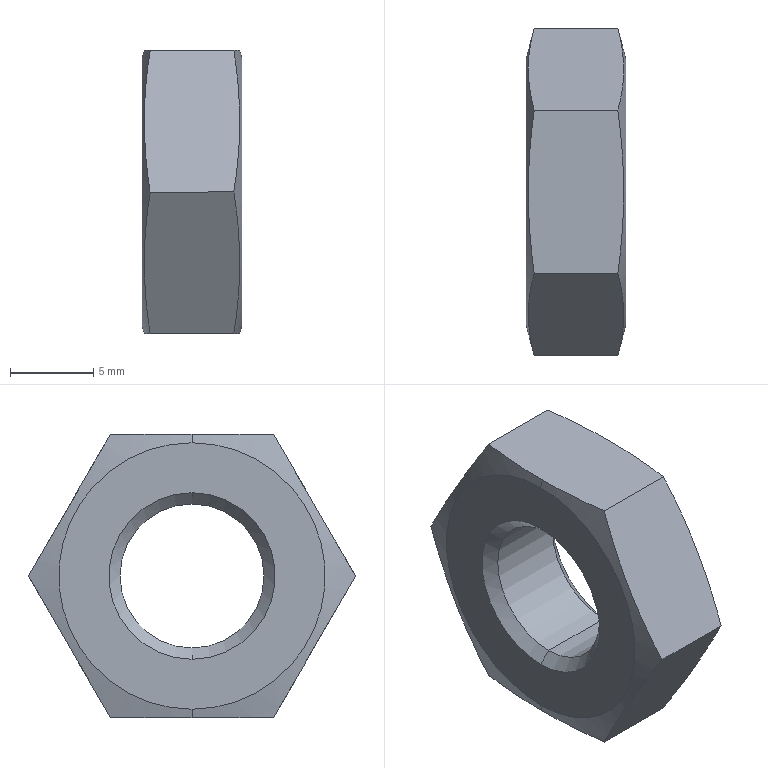Part | SolidWorks | features BaseBody 1 | 1 solid | 18 faces | box 6 x 19.63 x 17 mm | volume 1121 mm3 | cone 8 | plane 8 | cylinder 2 | commonest cylinder face diameters 8.647 x2
STEP:
#1=CARTESIAN_POINT('',(-2.324,0.,4.324));
#2=VERTEX_POINT('',#1);
#3=CARTESIAN_POINT('',(-2.324,0.,-4.324));
#4=VERTEX_POINT('',#3);
#5=CARTESIAN_POINT('',(-2.324,0.,0.));
#6=DIRECTION('',(1.,0.,0.));
#7=DIRECTION('',(0.,0.,-1.));
#8=AXIS2_PLACEMENT_3D('',#5,#6,#7);
#9=CIRCLE('',#8,4.324);
#10=EDGE_CURVE('',#2,#4,#9,.T.);
#11=ORIENTED_EDGE('',*,*,#10,.F.);
#12=CARTESIAN_POINT('',(2.324,0.,4.324));
#13=VERTEX_POINT('',#12);
#14=CARTESIAN_POINT('',(3.,0.,4.324));
#15=DIRECTION('',(1.,0.,0.));
#16=VECTOR('',#15,1000.);
#17=LINE('',#14,#16);
#18=EDGE_CURVE('',#2,#13,#17,.T.);
#19=ORIENTED_EDGE('',*,*,#18,.T.);
#20=CARTESIAN_POINT('',(2.324,0.,-4.324));
#21=VERTEX_POINT('',#20);
#22=CARTESIAN_POINT('',(2.324,0.,0.));
#23=DIRECTION('',(-1.,0.,0.));
#24=DIRECTION('',(0.,0.,-1.));
#25=AXIS2_PLACEMENT_3D('',#22,#23,#24);
#26=CIRCLE('',#25,4.324);
#27=EDGE_CURVE('',#21,#13,#26,.T.);
#28=ORIENTED_EDGE('',*,*,#27,.F.);
#29=CARTESIAN_POINT('',(3.,0.,-4.324));
#30=DIRECTION('',(1.,0.,0.));
#31=VECTOR('',#30,1000.);
#32=LINE('',#29,#31);
#33=EDGE_CURVE('',#4,#21,#32,.T.);
#34=ORIENTED_EDGE('',*,*,#33,.F.);
#35=EDGE_LOOP('',(#11,#19,#28,#34));
#36=FACE_OUTER_BOUND('',#35,.T.);
#37=CARTESIAN_POINT('',(3.,0.,0.));
#38=DIRECTION('',(1.,0.,0.));
#39=DIRECTION('',(0.,0.,-1.));
#40=AXIS2_PLACEMENT_3D('',#37,#38,#39);
#41=CYLINDRICAL_SURFACE('',#40,4.324);
#42=ADVANCED_FACE('',(#36),#41,.F.);
#43=ORIENTED_EDGE('',*,*,#10,.T.);
#44=CARTESIAN_POINT('',(-3.,0.,-5.));
#45=VERTEX_POINT('',#44);
#46=CARTESIAN_POINT('',(-3.,0.,-5.));
#47=DIRECTION('',(-0.7071,0.,-0.7071));
#48=VECTOR('',#47,1000.);
#49=LINE('',#46,#48);
#50=EDGE_CURVE('',#4,#45,#49,.T.);
#51=ORIENTED_EDGE('',*,*,#50,.T.);
#52=CARTESIAN_POINT('',(-3.,0.,5.));
#53=VERTEX_POINT('',#52);
#54=CARTESIAN_POINT('',(-3.,0.,0.));
#55=DIRECTION('',(1.,0.,0.));
#56=DIRECTION('',(0.,0.,1.));
#57=AXIS2_PLACEMENT_3D('',#54,#55,#56);
#58=CIRCLE('',#57,5.);
#59=EDGE_CURVE('',#53,#45,#58,.T.);
#60=ORIENTED_EDGE('',*,*,#59,.F.);
#61=CARTESIAN_POINT('',(-3.,0.,5.));
#62=DIRECTION('',(-0.7071,0.,0.7071));
#63=VECTOR('',#62,1000.);
#64=LINE('',#61,#63);
#65=EDGE_CURVE('',#2,#53,#64,.T.);
#66=ORIENTED_EDGE('',*,*,#65,.F.);
#67=EDGE_LOOP('',(#43,#51,#60,#66));
#68=FACE_OUTER_BOUND('',#67,.T.);
#69=CARTESIAN_POINT('',(-3.,0.,0.));
#70=DIRECTION('',(-1.,0.,0.));
#71=DIRECTION('',(0.,0.,1.));
#72=AXIS2_PLACEMENT_3D('',#69,#70,#71);
#73=CONICAL_SURFACE('',#72,5.,0.7854);
#74=ADVANCED_FACE('',(#68),#73,.F.);
#75=ORIENTED_EDGE('',*,*,#27,.T.);
#76=CARTESIAN_POINT('',(3.,0.,5.));
#77=VERTEX_POINT('',#76);
#78=CARTESIAN_POINT('',(3.,0.,5.));
#79=DIRECTION('',(0.7071,0.,0.7071));
#80=VECTOR('',#79,1000.);
#81=LINE('',#78,#80);
#82=EDGE_CURVE('',#13,#77,#81,.T.);
#83=ORIENTED_EDGE('',*,*,#82,.T.);
#84=CARTESIAN_POINT('',(3.,0.,-5.));
#85=VERTEX_POINT('',#84);
#86=CARTESIAN_POINT('',(3.,0.,0.));
#87=DIRECTION('',(-1.,0.,0.));
#88=DIRECTION('',(0.,0.,-1.));
#89=AXIS2_PLACEMENT_3D('',#86,#87,#88);
#90=CIRCLE('',#89,5.);
#91=EDGE_CURVE('',#85,#77,#90,.T.);
#92=ORIENTED_EDGE('',*,*,#91,.F.);
#93=CARTESIAN_POINT('',(3.,0.,-5.));
#94=DIRECTION('',(0.7071,0.,-0.7071));
#95=VECTOR('',#94,1000.);
#96=LINE('',#93,#95);
#97=EDGE_CURVE('',#21,#85,#96,.T.);
#98=ORIENTED_EDGE('',*,*,#97,.F.);
#99=EDGE_LOOP('',(#75,#83,#92,#98));
#100=FACE_OUTER_BOUND('',#99,.T.);
#101=CARTESIAN_POINT('',(3.,0.,0.));
#102=DIRECTION('',(1.,0.,0.));
#103=DIRECTION('',(0.,0.,-1.));
#104=AXIS2_PLACEMENT_3D('',#101,#102,#103);
#105=CONICAL_SURFACE('',#104,5.,0.7854);
#106=ADVANCED_FACE('',(#100),#105,.F.);
#107=CARTESIAN_POINT('',(-3.,0.,8.));
#108=VERTEX_POINT('',#107);
#109=CARTESIAN_POINT('',(-3.,0.,-8.));
#110=VERTEX_POINT('',#109);
#111=CARTESIAN_POINT('',(-3.,0.,0.));
#112=DIRECTION('',(-1.,0.,0.));
#113=DIRECTION('',(0.,0.,-1.));
#114=AXIS2_PLACEMENT_3D('',#111,#112,#113);
#115=CIRCLE('',#114,8.);
#116=EDGE_CURVE('',#108,#110,#115,.T.);
#117=ORIENTED_EDGE('',*,*,#116,.F.);
#118=CARTESIAN_POINT('',(-2.866,0.,8.5));
#119=VERTEX_POINT('',#118);
#120=CARTESIAN_POINT('',(-2.511,0.,9.826));
#121=DIRECTION('',(0.2588,0.,0.9659));
#122=VECTOR('',#121,1000.);
#123=LINE('',#120,#122);
#124=EDGE_CURVE('',#108,#119,#123,.T.);
#125=ORIENTED_EDGE('',*,*,#124,.T.);
#126=CARTESIAN_POINT('',(-2.514,4.907,8.5));
#127=VERTEX_POINT('',#126);
#128=CARTESIAN_POINT('',(-2.866,0.,8.5));
#129=CARTESIAN_POINT('',(-2.866,1.636,8.5));
#130=CARTESIAN_POINT('',(-2.733,3.272,8.5));
#131=CARTESIAN_POINT('',(-2.514,4.907,8.5));
#132=B_SPLINE_CURVE_WITH_KNOTS('',3,(#128,#129,#130,#131),.UNSPECIFIED.,.F.,.F.,(4,4),(0.004907,0.009815),.UNSPECIFIED.);
#133=EDGE_CURVE('',#119,#127,#132,.T.);
#134=ORIENTED_EDGE('',*,*,#133,.T.);
#135=CARTESIAN_POINT('',(-2.514,9.815,0.000000051));
#136=VERTEX_POINT('',#135);
#137=CARTESIAN_POINT('',(-2.514,4.907,8.5));
#138=CARTESIAN_POINT('',(-2.733,5.725,7.083));
#139=CARTESIAN_POINT('',(-2.999,7.361,4.25));
#140=CARTESIAN_POINT('',(-2.733,8.997,1.417));
#141=CARTESIAN_POINT('',(-2.514,9.815,0.000000051));
#142=B_SPLINE_CURVE_WITH_KNOTS('',3,(#137,#138,#139,#140,#141),.UNSPECIFIED.,.F.,.F.,(4,1,4),(0.,0.004907,0.009815),.UNSPECIFIED.);
#143=EDGE_CURVE('',#127,#136,#142,.T.);
#144=ORIENTED_EDGE('',*,*,#143,.T.);
#145=CARTESIAN_POINT('',(-2.514,4.907,-8.5));
#146=VERTEX_POINT('',#145);
#147=CARTESIAN_POINT('',(-2.514,9.815,0.000000051));
#148=CARTESIAN_POINT('',(-2.733,8.997,-1.417));
#149=CARTESIAN_POINT('',(-2.999,7.361,-4.25));
#150=CARTESIAN_POINT('',(-2.733,5.725,-7.083));
#151=CARTESIAN_POINT('',(-2.514,4.907,-8.5));
#152=B_SPLINE_CURVE_WITH_KNOTS('',3,(#147,#148,#149,#150,#151),.UNSPECIFIED.,.F.,.F.,(4,1,4),(0.,0.004907,0.009815),.UNSPECIFIED.);
#153=EDGE_CURVE('',#136,#146,#152,.T.);
#154=ORIENTED_EDGE('',*,*,#153,.T.);
#155=CARTESIAN_POINT('',(-2.866,0.,-8.5));
#156=VERTEX_POINT('',#155);
#157=CARTESIAN_POINT('',(-2.514,4.907,-8.5));
#158=CARTESIAN_POINT('',(-2.733,3.272,-8.5));
#159=CARTESIAN_POINT('',(-2.866,1.636,-8.5));
#160=CARTESIAN_POINT('',(-2.866,0.,-8.5));
#161=B_SPLINE_CURVE_WITH_KNOTS('',3,(#157,#158,#159,#160),.UNSPECIFIED.,.F.,.F.,(4,4),(0.,0.004907),.UNSPECIFIED.);
#162=EDGE_CURVE('',#146,#156,#161,.T.);
#163=ORIENTED_EDGE('',*,*,#162,.T.);
#164=CARTESIAN_POINT('',(-2.511,0.,-9.826));
#165=DIRECTION('',(0.2588,0.,-0.9659));
#166=VECTOR('',#165,1000.);
#167=LINE('',#164,#166);
#168=EDGE_CURVE('',#110,#156,#167,.T.);
#169=ORIENTED_EDGE('',*,*,#168,.F.);
#170=EDGE_LOOP('',(#117,#125,#134,#144,#154,#163,#169));
#171=FACE_OUTER_BOUND('',#170,.T.);
#172=CARTESIAN_POINT('',(-2.511,0.,0.));
#173=DIRECTION('',(1.,0.,0.));
#174=DIRECTION('',(0.,0.,-1.));
#175=AXIS2_PLACEMENT_3D('',#172,#173,#174);
#176=CONICAL_SURFACE('',#175,9.826,1.309);
#177=ADVANCED_FACE('',(#171),#176,.T.);
#178=CARTESIAN_POINT('',(3.,0.,-8.));
#179=VERTEX_POINT('',#178);
#180=CARTESIAN_POINT('',(3.,0.,8.));
#181=VERTEX_POINT('',#180);
#182=CARTESIAN_POINT('',(3.,0.,0.));
#183=DIRECTION('',(1.,0.,0.));
#184=DIRECTION('',(0.,0.,1.));
#185=AXIS2_PLACEMENT_3D('',#182,#183,#184);
#186=CIRCLE('',#185,8.);
#187=EDGE_CURVE('',#179,#181,#186,.T.);
#188=ORIENTED_EDGE('',*,*,#187,.F.);
#189=CARTESIAN_POINT('',(2.866,0.,-8.5));
#190=VERTEX_POINT('',#189);
#191=CARTESIAN_POINT('',(2.511,0.,-9.826));
#192=DIRECTION('',(-0.2588,0.,-0.9659));
#193=VECTOR('',#192,1000.);
#194=LINE('',#191,#193);
#195=EDGE_CURVE('',#179,#190,#194,.T.);
#196=ORIENTED_EDGE('',*,*,#195,.T.);
#197=CARTESIAN_POINT('',(2.514,4.907,-8.5));
#198=VERTEX_POINT('',#197);
#199=CARTESIAN_POINT('',(2.866,0.,-8.5));
#200=CARTESIAN_POINT('',(2.866,1.636,-8.5));
#201=CARTESIAN_POINT('',(2.733,3.272,-8.5));
#202=CARTESIAN_POINT('',(2.514,4.907,-8.5));
#203=B_SPLINE_CURVE_WITH_KNOTS('',3,(#199,#200,#201,#202),.UNSPECIFIED.,.F.,.F.,(4,4),(0.004907,0.009815),.UNSPECIFIED.);
#204=EDGE_CURVE('',#190,#198,#203,.T.);
#205=ORIENTED_EDGE('',*,*,#204,.T.);
#206=CARTESIAN_POINT('',(2.514,9.815,-0.000000051));
#207=VERTEX_POINT('',#206);
#208=CARTESIAN_POINT('',(2.514,4.907,-8.5));
#209=CARTESIAN_POINT('',(2.733,5.725,-7.083));
#210=CARTESIAN_POINT('',(2.999,7.361,-4.25));
#211=CARTESIAN_POINT('',(2.733,8.997,-1.417));
#212=CARTESIAN_POINT('',(2.514,9.815,-0.000000051));
#213=B_SPLINE_CURVE_WITH_KNOTS('',3,(#208,#209,#210,#211,#212),.UNSPECIFIED.,.F.,.F.,(4,1,4),(0.,0.004907,0.009815),.UNSPECIFIED.);
#214=EDGE_CURVE('',#198,#207,#213,.T.);
#215=ORIENTED_EDGE('',*,*,#214,.T.);
#216=CARTESIAN_POINT('',(2.514,4.907,8.5));
#217=VERTEX_POINT('',#216);
#218=CARTESIAN_POINT('',(2.514,9.815,-0.000000051));
#219=CARTESIAN_POINT('',(2.733,8.997,1.417));
#220=CARTESIAN_POINT('',(2.999,7.361,4.25));
#221=CARTESIAN_POINT('',(2.733,5.725,7.083));
#222=CARTESIAN_POINT('',(2.514,4.907,8.5));
#223=B_SPLINE_CURVE_WITH_KNOTS('',3,(#218,#219,#220,#221,#222),.UNSPECIFIED.,.F.,.F.,(4,1,4),(0.,0.004907,0.009815),.UNSPECIFIED.);
#224=EDGE_CURVE('',#207,#217,#223,.T.);
#225=ORIENTED_EDGE('',*,*,#224,.T.);
#226=CARTESIAN_POINT('',(2.866,0.,8.5));
#227=VERTEX_POINT('',#226);
#228=CARTESIAN_POINT('',(2.514,4.907,8.5));
#229=CARTESIAN_POINT('',(2.733,3.272,8.5));
#230=CARTESIAN_POINT('',(2.866,1.636,8.5));
#231=CARTESIAN_POINT('',(2.866,0.,8.5));
#232=B_SPLINE_CURVE_WITH_KNOTS('',3,(#228,#229,#230,#231),.UNSPECIFIED.,.F.,.F.,(4,4),(0.,0.004907),.UNSPECIFIED.);
#233=EDGE_CURVE('',#217,#227,#232,.T.);
#234=ORIENTED_EDGE('',*,*,#233,.T.);
#235=CARTESIAN_POINT('',(2.511,0.,9.826));
#236=DIRECTION('',(-0.2588,0.,0.9659));
#237=VECTOR('',#236,1000.);
#238=LINE('',#235,#237);
#239=EDGE_CURVE('',#181,#227,#238,.T.);
#240=ORIENTED_EDGE('',*,*,#239,.F.);
#241=EDGE_LOOP('',(#188,#196,#205,#215,#225,#234,#240));
#242=FACE_OUTER_BOUND('',#241,.T.);
#243=CARTESIAN_POINT('',(2.511,0.,0.));
#244=DIRECTION('',(-1.,0.,0.));
#245=DIRECTION('',(0.,0.,1.));
#246=AXIS2_PLACEMENT_3D('',#243,#244,#245);
#247=CONICAL_SURFACE('',#246,9.826,1.309);
#248=ADVANCED_FACE('',(#242),#247,.T.);
#249=ORIENTED_EDGE('',*,*,#18,.F.);
#250=CARTESIAN_POINT('',(-2.324,0.,0.));
#251=DIRECTION('',(1.,0.,0.));
#252=DIRECTION('',(0.,0.,-1.));
#253=AXIS2_PLACEMENT_3D('',#250,#251,#252);
#254=CIRCLE('',#253,4.324);
#255=EDGE_CURVE('',#4,#2,#254,.T.);
#256=ORIENTED_EDGE('',*,*,#255,.F.);
#257=ORIENTED_EDGE('',*,*,#33,.T.);
#258=CARTESIAN_POINT('',(2.324,0.,0.));
#259=DIRECTION('',(-1.,0.,0.));
#260=DIRECTION('',(0.,0.,-1.));
#261=AXIS2_PLACEMENT_3D('',#258,#259,#260);
#262=CIRCLE('',#261,4.324);
#263=EDGE_CURVE('',#13,#21,#262,.T.);
#264=ORIENTED_EDGE('',*,*,#263,.F.);
#265=EDGE_LOOP('',(#249,#256,#257,#264));
#266=FACE_OUTER_BOUND('',#265,.T.);
#267=CARTESIAN_POINT('',(3.,0.,0.));
#268=DIRECTION('',(1.,0.,0.));
#269=DIRECTION('',(0.,0.,-1.));
#270=AXIS2_PLACEMENT_3D('',#267,#268,#269);
#271=CYLINDRICAL_SURFACE('',#270,4.324);
#272=ADVANCED_FACE('',(#266),#271,.F.);
#273=ORIENTED_EDGE('',*,*,#50,.F.);
#274=ORIENTED_EDGE('',*,*,#255,.T.);
#275=ORIENTED_EDGE('',*,*,#65,.T.);
#276=CARTESIAN_POINT('',(-3.,0.,0.));
#277=DIRECTION('',(1.,0.,0.));
#278=DIRECTION('',(0.,0.,1.));
#279=AXIS2_PLACEMENT_3D('',#276,#277,#278);
#280=CIRCLE('',#279,5.);
#281=EDGE_CURVE('',#45,#53,#280,.T.);
#282=ORIENTED_EDGE('',*,*,#281,.F.);
#283=EDGE_LOOP('',(#273,#274,#275,#282));
#284=FACE_OUTER_BOUND('',#283,.T.);
#285=CARTESIAN_POINT('',(-3.,0.,0.));
#286=DIRECTION('',(-1.,0.,0.));
#287=DIRECTION('',(0.,0.,1.));
#288=AXIS2_PLACEMENT_3D('',#285,#286,#287);
#289=CONICAL_SURFACE('',#288,5.,0.7854);
#290=ADVANCED_FACE('',(#284),#289,.F.);
#291=ORIENTED_EDGE('',*,*,#82,.F.);
#292=ORIENTED_EDGE('',*,*,#263,.T.);
#293=ORIENTED_EDGE('',*,*,#97,.T.);
#294=CARTESIAN_POINT('',(3.,0.,0.));
#295=DIRECTION('',(-1.,0.,0.));
#296=DIRECTION('',(0.,0.,-1.));
#297=AXIS2_PLACEMENT_3D('',#294,#295,#296);
#298=CIRCLE('',#297,5.);
#299=EDGE_CURVE('',#77,#85,#298,.T.);
#300=ORIENTED_EDGE('',*,*,#299,.F.);
#301=EDGE_LOOP('',(#291,#292,#293,#300));
#302=FACE_OUTER_BOUND('',#301,.T.);
#303=CARTESIAN_POINT('',(3.,0.,0.));
#304=DIRECTION('',(1.,0.,0.));
#305=DIRECTION('',(0.,0.,-1.));
#306=AXIS2_PLACEMENT_3D('',#303,#304,#305);
#307=CONICAL_SURFACE('',#306,5.,0.7854);
#308=ADVANCED_FACE('',(#302),#307,.F.);
#309=CARTESIAN_POINT('',(-3.,0.,0.));
#310=DIRECTION('',(-1.,0.,0.));
#311=DIRECTION('',(0.,0.,-1.));
#312=AXIS2_PLACEMENT_3D('',#309,#310,#311);
#313=CIRCLE('',#312,8.);
#314=EDGE_CURVE('',#110,#108,#313,.T.);
#315=ORIENTED_EDGE('',*,*,#314,.T.);
#316=ORIENTED_EDGE('',*,*,#116,.T.);
#317=EDGE_LOOP('',(#315,#316));
#318=FACE_OUTER_BOUND('',#317,.T.);
#319=ORIENTED_EDGE('',*,*,#59,.T.);
#320=ORIENTED_EDGE('',*,*,#281,.T.);
#321=EDGE_LOOP('',(#319,#320));
#322=FACE_BOUND('',#321,.T.);
#323=CARTESIAN_POINT('',(-3.,8.,0.));
#324=DIRECTION('',(-1.,0.,0.));
#325=DIRECTION('',(0.,0.,1.));
#326=AXIS2_PLACEMENT_3D('',#323,#324,#325);
#327=PLANE('',#326);
#328=ADVANCED_FACE('',(#318,#322),#327,.T.);
#329=ORIENTED_EDGE('',*,*,#91,.T.);
#330=ORIENTED_EDGE('',*,*,#299,.T.);
#331=EDGE_LOOP('',(#329,#330));
#332=FACE_BOUND('',#331,.T.);
#333=CARTESIAN_POINT('',(3.,0.,0.));
#334=DIRECTION('',(1.,0.,0.));
#335=DIRECTION('',(0.,0.,1.));
#336=AXIS2_PLACEMENT_3D('',#333,#334,#335);
#337=CIRCLE('',#336,8.);
#338=EDGE_CURVE('',#181,#179,#337,.T.);
#339=ORIENTED_EDGE('',*,*,#338,.T.);
#340=ORIENTED_EDGE('',*,*,#187,.T.);
#341=EDGE_LOOP('',(#339,#340));
#342=FACE_OUTER_BOUND('',#341,.T.);
#343=CARTESIAN_POINT('',(3.,5.,0.));
#344=DIRECTION('',(1.,0.,0.));
#345=DIRECTION('',(0.,0.,-1.));
#346=AXIS2_PLACEMENT_3D('',#343,#344,#345);
#347=PLANE('',#346);
#348=ADVANCED_FACE('',(#332,#342),#347,.T.);
#349=ORIENTED_EDGE('',*,*,#124,.F.);
#350=ORIENTED_EDGE('',*,*,#314,.F.);
#351=ORIENTED_EDGE('',*,*,#168,.T.);
#352=CARTESIAN_POINT('',(-2.514,-4.907,-8.5));
#353=VERTEX_POINT('',#352);
#354=CARTESIAN_POINT('',(-2.866,0.,-8.5));
#355=CARTESIAN_POINT('',(-2.866,-1.636,-8.5));
#356=CARTESIAN_POINT('',(-2.733,-3.272,-8.5));
#357=CARTESIAN_POINT('',(-2.514,-4.907,-8.5));
#358=B_SPLINE_CURVE_WITH_KNOTS('',3,(#354,#355,#356,#357),.UNSPECIFIED.,.F.,.F.,(4,4),(0.004907,0.009815),.UNSPECIFIED.);
#359=EDGE_CURVE('',#156,#353,#358,.T.);
#360=ORIENTED_EDGE('',*,*,#359,.T.);
#361=CARTESIAN_POINT('',(-2.514,-9.815,-0.000000051));
#362=VERTEX_POINT('',#361);
#363=CARTESIAN_POINT('',(-2.514,-4.907,-8.5));
#364=CARTESIAN_POINT('',(-2.733,-5.725,-7.083));
#365=CARTESIAN_POINT('',(-2.999,-7.361,-4.25));
#366=CARTESIAN_POINT('',(-2.733,-8.997,-1.417));
#367=CARTESIAN_POINT('',(-2.514,-9.815,-0.000000051));
#368=B_SPLINE_CURVE_WITH_KNOTS('',3,(#363,#364,#365,#366,#367),.UNSPECIFIED.,.F.,.F.,(4,1,4),(0.,0.004907,0.009815),.UNSPECIFIED.);
#369=EDGE_CURVE('',#353,#362,#368,.T.);
#370=ORIENTED_EDGE('',*,*,#369,.T.);
#371=CARTESIAN_POINT('',(-2.514,-4.907,8.5));
#372=VERTEX_POINT('',#371);
#373=CARTESIAN_POINT('',(-2.514,-9.815,-0.000000051));
#374=CARTESIAN_POINT('',(-2.733,-8.997,1.417));
#375=CARTESIAN_POINT('',(-2.999,-7.361,4.25));
#376=CARTESIAN_POINT('',(-2.733,-5.725,7.083));
#377=CARTESIAN_POINT('',(-2.514,-4.907,8.5));
#378=B_SPLINE_CURVE_WITH_KNOTS('',3,(#373,#374,#375,#376,#377),.UNSPECIFIED.,.F.,.F.,(4,1,4),(0.,0.004907,0.009815),.UNSPECIFIED.);
#379=EDGE_CURVE('',#362,#372,#378,.T.);
#380=ORIENTED_EDGE('',*,*,#379,.T.);
#381=CARTESIAN_POINT('',(-2.514,-4.907,8.5));
#382=CARTESIAN_POINT('',(-2.733,-3.272,8.5));
#383=CARTESIAN_POINT('',(-2.866,-1.636,8.5));
#384=CARTESIAN_POINT('',(-2.866,0.,8.5));
#385=B_SPLINE_CURVE_WITH_KNOTS('',3,(#381,#382,#383,#384),.UNSPECIFIED.,.F.,.F.,(4,4),(0.,0.004907),.UNSPECIFIED.);
#386=EDGE_CURVE('',#372,#119,#385,.T.);
#387=ORIENTED_EDGE('',*,*,#386,.T.);
#388=EDGE_LOOP('',(#349,#350,#351,#360,#370,#380,#387));
#389=FACE_OUTER_BOUND('',#388,.T.);
#390=CARTESIAN_POINT('',(-2.511,0.,0.));
#391=DIRECTION('',(1.,0.,0.));
#392=DIRECTION('',(0.,0.,-1.));
#393=AXIS2_PLACEMENT_3D('',#390,#391,#392);
#394=CONICAL_SURFACE('',#393,9.826,1.309);
#395=ADVANCED_FACE('',(#389),#394,.T.);
#396=ORIENTED_EDGE('',*,*,#195,.F.);
#397=ORIENTED_EDGE('',*,*,#338,.F.);
#398=ORIENTED_EDGE('',*,*,#239,.T.);
#399=CARTESIAN_POINT('',(2.514,-4.907,8.5));
#400=VERTEX_POINT('',#399);
#401=CARTESIAN_POINT('',(2.866,0.,8.5));
#402=CARTESIAN_POINT('',(2.866,-1.636,8.5));
#403=CARTESIAN_POINT('',(2.733,-3.272,8.5));
#404=CARTESIAN_POINT('',(2.514,-4.907,8.5));
#405=B_SPLINE_CURVE_WITH_KNOTS('',3,(#401,#402,#403,#404),.UNSPECIFIED.,.F.,.F.,(4,4),(0.004907,0.009815),.UNSPECIFIED.);
#406=EDGE_CURVE('',#227,#400,#405,.T.);
#407=ORIENTED_EDGE('',*,*,#406,.T.);
#408=CARTESIAN_POINT('',(2.514,-9.815,0.000000051));
#409=VERTEX_POINT('',#408);
#410=CARTESIAN_POINT('',(2.514,-4.907,8.5));
#411=CARTESIAN_POINT('',(2.733,-5.725,7.083));
#412=CARTESIAN_POINT('',(2.999,-7.361,4.25));
#413=CARTESIAN_POINT('',(2.733,-8.997,1.417));
#414=CARTESIAN_POINT('',(2.514,-9.815,0.000000051));
#415=B_SPLINE_CURVE_WITH_KNOTS('',3,(#410,#411,#412,#413,#414),.UNSPECIFIED.,.F.,.F.,(4,1,4),(0.,0.004907,0.009815),.UNSPECIFIED.);
#416=EDGE_CURVE('',#400,#409,#415,.T.);
#417=ORIENTED_EDGE('',*,*,#416,.T.);
#418=CARTESIAN_POINT('',(2.514,-4.907,-8.5));
#419=VERTEX_POINT('',#418);
#420=CARTESIAN_POINT('',(2.514,-9.815,0.000000051));
#421=CARTESIAN_POINT('',(2.733,-8.997,-1.417));
#422=CARTESIAN_POINT('',(2.999,-7.361,-4.25));
#423=CARTESIAN_POINT('',(2.733,-5.725,-7.083));
#424=CARTESIAN_POINT('',(2.514,-4.907,-8.5));
#425=B_SPLINE_CURVE_WITH_KNOTS('',3,(#420,#421,#422,#423,#424),.UNSPECIFIED.,.F.,.F.,(4,1,4),(0.,0.004907,0.009815),.UNSPECIFIED.);
#426=EDGE_CURVE('',#409,#419,#425,.T.);
#427=ORIENTED_EDGE('',*,*,#426,.T.);
#428=CARTESIAN_POINT('',(2.514,-4.907,-8.5));
#429=CARTESIAN_POINT('',(2.733,-3.272,-8.5));
#430=CARTESIAN_POINT('',(2.866,-1.636,-8.5));
#431=CARTESIAN_POINT('',(2.866,0.,-8.5));
#432=B_SPLINE_CURVE_WITH_KNOTS('',3,(#428,#429,#430,#431),.UNSPECIFIED.,.F.,.F.,(4,4),(0.,0.004907),.UNSPECIFIED.);
#433=EDGE_CURVE('',#419,#190,#432,.T.);
#434=ORIENTED_EDGE('',*,*,#433,.T.);
#435=EDGE_LOOP('',(#396,#397,#398,#407,#417,#427,#434));
#436=FACE_OUTER_BOUND('',#435,.T.);
#437=CARTESIAN_POINT('',(2.511,0.,0.));
#438=DIRECTION('',(-1.,0.,0.));
#439=DIRECTION('',(0.,0.,1.));
#440=AXIS2_PLACEMENT_3D('',#437,#438,#439);
#441=CONICAL_SURFACE('',#440,9.826,1.309);
#442=ADVANCED_FACE('',(#436),#441,.T.);
#443=CARTESIAN_POINT('',(3.,-9.815,0.));
#444=DIRECTION('',(-1.,0.,0.));
#445=VECTOR('',#444,1000.);
#446=LINE('',#443,#445);
#447=EDGE_CURVE('',#409,#362,#446,.T.);
#448=ORIENTED_EDGE('',*,*,#447,.F.);
#449=ORIENTED_EDGE('',*,*,#416,.F.);
#450=CARTESIAN_POINT('',(3.,-4.907,8.5));
#451=DIRECTION('',(1.,0.,0.));
#452=VECTOR('',#451,1000.);
#453=LINE('',#450,#452);
#454=EDGE_CURVE('',#372,#400,#453,.T.);
#455=ORIENTED_EDGE('',*,*,#454,.F.);
#456=ORIENTED_EDGE('',*,*,#379,.F.);
#457=EDGE_LOOP('',(#448,#449,#455,#456));
#458=FACE_OUTER_BOUND('',#457,.T.);
#459=CARTESIAN_POINT('',(3.,-4.907,8.5));
#460=DIRECTION('',(0.,0.866,-0.5));
#461=DIRECTION('',(0.,0.5,0.866));
#462=AXIS2_PLACEMENT_3D('',#459,#460,#461);
#463=PLANE('',#462);
#464=ADVANCED_FACE('',(#458),#463,.F.);
#465=CARTESIAN_POINT('',(3.,-4.907,-8.5));
#466=DIRECTION('',(-1.,0.,0.));
#467=VECTOR('',#466,1000.);
#468=LINE('',#465,#467);
#469=EDGE_CURVE('',#419,#353,#468,.T.);
#470=ORIENTED_EDGE('',*,*,#469,.F.);
#471=ORIENTED_EDGE('',*,*,#426,.F.);
#472=ORIENTED_EDGE('',*,*,#447,.T.);
#473=ORIENTED_EDGE('',*,*,#369,.F.);
#474=EDGE_LOOP('',(#470,#471,#472,#473));
#475=FACE_OUTER_BOUND('',#474,.T.);
#476=CARTESIAN_POINT('',(3.,-9.815,0.));
#477=DIRECTION('',(0.,0.866,0.5));
#478=DIRECTION('',(0.,-0.5,0.866));
#479=AXIS2_PLACEMENT_3D('',#476,#477,#478);
#480=PLANE('',#479);
#481=ADVANCED_FACE('',(#475),#480,.F.);
#482=CARTESIAN_POINT('',(3.,4.907,-8.5));
#483=DIRECTION('',(-1.,0.,0.));
#484=VECTOR('',#483,1000.);
#485=LINE('',#482,#484);
#486=EDGE_CURVE('',#198,#146,#485,.T.);
#487=ORIENTED_EDGE('',*,*,#486,.F.);
#488=ORIENTED_EDGE('',*,*,#204,.F.);
#489=ORIENTED_EDGE('',*,*,#433,.F.);
#490=ORIENTED_EDGE('',*,*,#469,.T.);
#491=ORIENTED_EDGE('',*,*,#359,.F.);
#492=ORIENTED_EDGE('',*,*,#162,.F.);
#493=EDGE_LOOP('',(#487,#488,#489,#490,#491,#492));
#494=FACE_OUTER_BOUND('',#493,.T.);
#495=CARTESIAN_POINT('',(3.,-4.907,-8.5));
#496=DIRECTION('',(0.,0.,1.));
#497=DIRECTION('',(1.,0.,0.));
#498=AXIS2_PLACEMENT_3D('',#495,#496,#497);
#499=PLANE('',#498);
#500=ADVANCED_FACE('',(#494),#499,.F.);
#501=CARTESIAN_POINT('',(3.,9.815,0.));
#502=DIRECTION('',(-1.,0.,0.));
#503=VECTOR('',#502,1000.);
#504=LINE('',#501,#503);
#505=EDGE_CURVE('',#207,#136,#504,.T.);
#506=ORIENTED_EDGE('',*,*,#505,.F.);
#507=ORIENTED_EDGE('',*,*,#214,.F.);
#508=ORIENTED_EDGE('',*,*,#486,.T.);
#509=ORIENTED_EDGE('',*,*,#153,.F.);
#510=EDGE_LOOP('',(#506,#507,#508,#509));
#511=FACE_OUTER_BOUND('',#510,.T.);
#512=CARTESIAN_POINT('',(3.,4.907,-8.5));
#513=DIRECTION('',(0.,-0.866,0.5));
#514=DIRECTION('',(0.,-0.5,-0.866));
#515=AXIS2_PLACEMENT_3D('',#512,#513,#514);
#516=PLANE('',#515);
#517=ADVANCED_FACE('',(#511),#516,.F.);
#518=CARTESIAN_POINT('',(3.,4.907,8.5));
#519=DIRECTION('',(-1.,0.,0.));
#520=VECTOR('',#519,1000.);
#521=LINE('',#518,#520);
#522=EDGE_CURVE('',#217,#127,#521,.T.);
#523=ORIENTED_EDGE('',*,*,#522,.F.);
#524=ORIENTED_EDGE('',*,*,#224,.F.);
#525=ORIENTED_EDGE('',*,*,#505,.T.);
#526=ORIENTED_EDGE('',*,*,#143,.F.);
#527=EDGE_LOOP('',(#523,#524,#525,#526));
#528=FACE_OUTER_BOUND('',#527,.T.);
#529=CARTESIAN_POINT('',(3.,9.815,0.));
#530=DIRECTION('',(0.,-0.866,-0.5));
#531=DIRECTION('',(0.,0.5,-0.866));
#532=AXIS2_PLACEMENT_3D('',#529,#530,#531);
#533=PLANE('',#532);
#534=ADVANCED_FACE('',(#528),#533,.F.);
#535=ORIENTED_EDGE('',*,*,#454,.T.);
#536=ORIENTED_EDGE('',*,*,#406,.F.);
#537=ORIENTED_EDGE('',*,*,#233,.F.);
#538=ORIENTED_EDGE('',*,*,#522,.T.);
#539=ORIENTED_EDGE('',*,*,#133,.F.);
#540=ORIENTED_EDGE('',*,*,#386,.F.);
#541=EDGE_LOOP('',(#535,#536,#537,#538,#539,#540));
#542=FACE_OUTER_BOUND('',#541,.T.);
#543=CARTESIAN_POINT('',(3.,4.907,8.5));
#544=DIRECTION('',(0.,0.,-1.));
#545=DIRECTION('',(-1.,0.,0.));
#546=AXIS2_PLACEMENT_3D('',#543,#544,#545);
#547=PLANE('',#546);
#548=ADVANCED_FACE('',(#542),#547,.F.);
#549=CLOSED_SHELL('',(#42,#74,#106,#177,#248,#272,#290,#308,#328,#348,#395,#442,#464,#481,#500,#517,#534,#548));
#550=MANIFOLD_SOLID_BREP('',#549);
#551=CARTESIAN_POINT('',(0.,0.,0.));
#552=DIRECTION('',(0.,0.,1.));
#553=DIRECTION('',(1.,0.,0.));
#554=AXIS2_PLACEMENT_3D('',#551,#552,#553);
#555=(LENGTH_UNIT()NAMED_UNIT(*)SI_UNIT(.MILLI.,.METRE.));
#556=UNCERTAINTY_MEASURE_WITH_UNIT(LENGTH_MEASURE(0.00001),#555,'','');
#557=(NAMED_UNIT(*)PLANE_ANGLE_UNIT()SI_UNIT($,.RADIAN.));
#558=(NAMED_UNIT(*)SI_UNIT($,.STERADIAN.)SOLID_ANGLE_UNIT());
#559=(GEOMETRIC_REPRESENTATION_CONTEXT(3)GLOBAL_UNCERTAINTY_ASSIGNED_CONTEXT((#556))GLOBAL_UNIT_ASSIGNED_CONTEXT((#555,#557,#558))REPRESENTATION_CONTEXT('',''));
#560=ADVANCED_BREP_SHAPE_REPRESENTATION('',(#550,#554),#559);